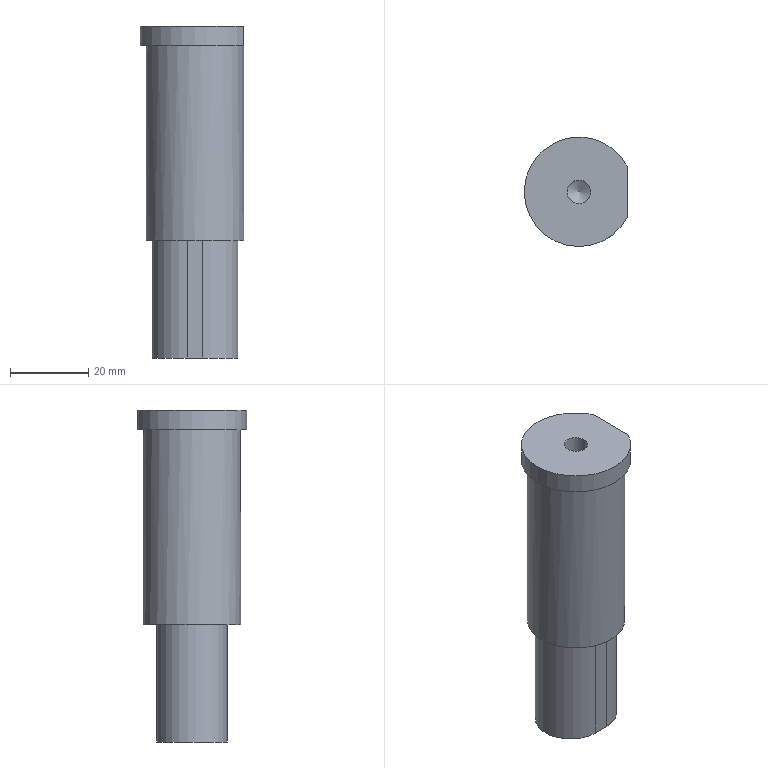Part | NX | features solid 2 | 1 solid | 15 faces | box 26.5 x 28 x 85 mm | volume 36969 mm3 | plane 7 | cylinder 7 | cone 1 | commonest cylinder face diameters 28 x3 18 x2 6 x1 25 x1
STEP:
#1=CARTESIAN_POINT('',(-212.5,0.005131,75.));
#2=VERTEX_POINT('',#1);
#3=CARTESIAN_POINT('',(-212.5,6.31,75.));
#4=VERTEX_POINT('',#3);
#5=CARTESIAN_POINT('',(-212.5,-22.334,75.));
#6=DIRECTION('',(0.,1.,0.));
#7=VECTOR('',#6,1000.);
#8=LINE('',#5,#7);
#9=EDGE_CURVE('',#2,#4,#8,.T.);
#10=ORIENTED_EDGE('',*,*,#9,.F.);
#11=CARTESIAN_POINT('',(-225.,0.005131,75.));
#12=DIRECTION('',(0.,0.,1.));
#13=DIRECTION('',(0.,-1.,0.));
#14=AXIS2_PLACEMENT_3D('',#11,#12,#13);
#15=CIRCLE('',#14,12.5);
#16=EDGE_CURVE('',#2,#2,#15,.T.);
#17=ORIENTED_EDGE('',*,*,#16,.T.);
#18=CARTESIAN_POINT('',(-212.5,-6.3,75.));
#19=VERTEX_POINT('',#18);
#20=CARTESIAN_POINT('',(-212.5,-22.334,75.));
#21=DIRECTION('',(0.,1.,0.));
#22=VECTOR('',#21,1000.);
#23=LINE('',#20,#22);
#24=EDGE_CURVE('',#19,#2,#23,.T.);
#25=ORIENTED_EDGE('',*,*,#24,.F.);
#26=CARTESIAN_POINT('',(-231.305,12.505,75.));
#27=VERTEX_POINT('',#26);
#28=CARTESIAN_POINT('',(-225.,0.005131,75.));
#29=DIRECTION('',(0.,0.,1.));
#30=DIRECTION('',(0.,-1.,0.));
#31=AXIS2_PLACEMENT_3D('',#28,#29,#30);
#32=CIRCLE('',#31,14.);
#33=EDGE_CURVE('',#27,#19,#32,.T.);
#34=ORIENTED_EDGE('',*,*,#33,.F.);
#35=CARTESIAN_POINT('',(-218.695,12.505,75.));
#36=VERTEX_POINT('',#35);
#37=CARTESIAN_POINT('',(-225.,0.005131,75.));
#38=DIRECTION('',(0.,0.,1.));
#39=DIRECTION('',(1.,0.,0.));
#40=AXIS2_PLACEMENT_3D('',#37,#38,#39);
#41=CIRCLE('',#40,14.);
#42=EDGE_CURVE('',#27,#36,#41,.F.);
#43=ORIENTED_EDGE('',*,*,#42,.T.);
#44=CARTESIAN_POINT('',(-225.,0.005131,75.));
#45=DIRECTION('',(0.,0.,1.));
#46=DIRECTION('',(0.,-1.,0.));
#47=AXIS2_PLACEMENT_3D('',#44,#45,#46);
#48=CIRCLE('',#47,14.);
#49=EDGE_CURVE('',#4,#36,#48,.T.);
#50=ORIENTED_EDGE('',*,*,#49,.F.);
#51=EDGE_LOOP('',(#10,#17,#25,#34,#43,#50));
#52=FACE_BOUND('',#51,.T.);
#53=CARTESIAN_POINT('',(-225.,0.005131,75.));
#54=DIRECTION('',(0.,0.,1.));
#55=DIRECTION('',(0.,-1.,0.));
#56=AXIS2_PLACEMENT_3D('',#53,#54,#55);
#57=PLANE('',#56);
#58=ADVANCED_FACE('',(#52),#57,.F.);
#59=CARTESIAN_POINT('',(-212.5,6.31,80.));
#60=VERTEX_POINT('',#59);
#61=CARTESIAN_POINT('',(-218.695,12.505,80.));
#62=VERTEX_POINT('',#61);
#63=CARTESIAN_POINT('',(-225.,0.005131,80.));
#64=DIRECTION('',(0.,0.,1.));
#65=DIRECTION('',(0.,-1.,0.));
#66=AXIS2_PLACEMENT_3D('',#63,#64,#65);
#67=CIRCLE('',#66,14.);
#68=EDGE_CURVE('',#60,#62,#67,.T.);
#69=ORIENTED_EDGE('',*,*,#68,.F.);
#70=CARTESIAN_POINT('',(-212.5,6.31,75.));
#71=DIRECTION('',(0.,0.,1.));
#72=VECTOR('',#71,1000.);
#73=LINE('',#70,#72);
#74=EDGE_CURVE('',#60,#4,#73,.F.);
#75=ORIENTED_EDGE('',*,*,#74,.T.);
#76=ORIENTED_EDGE('',*,*,#49,.T.);
#77=CARTESIAN_POINT('',(-218.695,12.505,83.));
#78=DIRECTION('',(0.,0.,-1.));
#79=VECTOR('',#78,1000.);
#80=LINE('',#77,#79);
#81=EDGE_CURVE('',#62,#36,#80,.T.);
#82=ORIENTED_EDGE('',*,*,#81,.F.);
#83=EDGE_LOOP('',(#69,#75,#76,#82));
#84=FACE_BOUND('',#83,.T.);
#85=CARTESIAN_POINT('',(-225.,0.005131,75.));
#86=DIRECTION('',(0.,0.,1.));
#87=DIRECTION('',(0.,-1.,0.));
#88=AXIS2_PLACEMENT_3D('',#85,#86,#87);
#89=CYLINDRICAL_SURFACE('',#88,14.);
#90=ADVANCED_FACE('',(#84),#89,.T.);
#91=ORIENTED_EDGE('',*,*,#33,.T.);
#92=CARTESIAN_POINT('',(-212.5,-6.3,80.));
#93=VERTEX_POINT('',#92);
#94=CARTESIAN_POINT('',(-212.5,-6.3,75.));
#95=DIRECTION('',(0.,0.,1.));
#96=VECTOR('',#95,1000.);
#97=LINE('',#94,#96);
#98=EDGE_CURVE('',#19,#93,#97,.T.);
#99=ORIENTED_EDGE('',*,*,#98,.T.);
#100=CARTESIAN_POINT('',(-231.305,12.505,80.));
#101=VERTEX_POINT('',#100);
#102=CARTESIAN_POINT('',(-225.,0.005131,80.));
#103=DIRECTION('',(0.,0.,1.));
#104=DIRECTION('',(0.,-1.,0.));
#105=AXIS2_PLACEMENT_3D('',#102,#103,#104);
#106=CIRCLE('',#105,14.);
#107=EDGE_CURVE('',#101,#93,#106,.T.);
#108=ORIENTED_EDGE('',*,*,#107,.F.);
#109=CARTESIAN_POINT('',(-231.305,12.505,83.));
#110=DIRECTION('',(0.,0.,-1.));
#111=VECTOR('',#110,1000.);
#112=LINE('',#109,#111);
#113=EDGE_CURVE('',#101,#27,#112,.T.);
#114=ORIENTED_EDGE('',*,*,#113,.T.);
#115=EDGE_LOOP('',(#91,#99,#108,#114));
#116=FACE_BOUND('',#115,.T.);
#117=CARTESIAN_POINT('',(-225.,0.005131,75.));
#118=DIRECTION('',(0.,0.,1.));
#119=DIRECTION('',(0.,-1.,0.));
#120=AXIS2_PLACEMENT_3D('',#117,#118,#119);
#121=CYLINDRICAL_SURFACE('',#120,14.);
#122=ADVANCED_FACE('',(#116),#121,.T.);
#123=CARTESIAN_POINT('',(-225.,3.005,80.));
#124=VERTEX_POINT('',#123);
#125=CARTESIAN_POINT('',(-225.,0.005131,80.));
#126=DIRECTION('',(0.,0.,-1.));
#127=DIRECTION('',(0.,1.,0.));
#128=AXIS2_PLACEMENT_3D('',#125,#126,#127);
#129=CIRCLE('',#128,3.);
#130=EDGE_CURVE('',#124,#124,#129,.T.);
#131=ORIENTED_EDGE('',*,*,#130,.T.);
#132=EDGE_LOOP('',(#131));
#133=FACE_BOUND('',#132,.T.);
#134=ORIENTED_EDGE('',*,*,#107,.T.);
#135=CARTESIAN_POINT('',(-212.5,-22.334,80.));
#136=DIRECTION('',(0.,1.,0.));
#137=VECTOR('',#136,1000.);
#138=LINE('',#135,#137);
#139=EDGE_CURVE('',#93,#60,#138,.T.);
#140=ORIENTED_EDGE('',*,*,#139,.T.);
#141=ORIENTED_EDGE('',*,*,#68,.T.);
#142=CARTESIAN_POINT('',(-225.,0.005131,80.));
#143=DIRECTION('',(0.,0.,1.));
#144=DIRECTION('',(1.,0.,0.));
#145=AXIS2_PLACEMENT_3D('',#142,#143,#144);
#146=CIRCLE('',#145,14.);
#147=EDGE_CURVE('',#101,#62,#146,.F.);
#148=ORIENTED_EDGE('',*,*,#147,.F.);
#149=EDGE_LOOP('',(#134,#140,#141,#148));
#150=FACE_BOUND('',#149,.T.);
#151=CARTESIAN_POINT('',(-225.,0.005131,80.));
#152=DIRECTION('',(0.,0.,1.));
#153=DIRECTION('',(0.,-1.,0.));
#154=AXIS2_PLACEMENT_3D('',#151,#152,#153);
#155=PLANE('',#154);
#156=ADVANCED_FACE('',(#133,#150),#155,.T.);
#157=CARTESIAN_POINT('',(-225.,-12.495,25.));
#158=VERTEX_POINT('',#157);
#159=CARTESIAN_POINT('',(-225.,0.005131,25.));
#160=DIRECTION('',(0.,0.,1.));
#161=DIRECTION('',(0.,-1.,0.));
#162=AXIS2_PLACEMENT_3D('',#159,#160,#161);
#163=CIRCLE('',#162,12.5);
#164=EDGE_CURVE('',#158,#158,#163,.T.);
#165=ORIENTED_EDGE('',*,*,#164,.F.);
#166=EDGE_LOOP('',(#165));
#167=FACE_BOUND('',#166,.T.);
#168=CARTESIAN_POINT('',(-223.,-8.995,25.));
#169=VERTEX_POINT('',#168);
#170=CARTESIAN_POINT('',(-227.,-8.995,25.));
#171=VERTEX_POINT('',#170);
#172=CARTESIAN_POINT('',(-225.,-8.995,25.));
#173=DIRECTION('',(-1.,0.,0.));
#174=VECTOR('',#173,1000.);
#175=LINE('',#172,#174);
#176=EDGE_CURVE('',#169,#171,#175,.T.);
#177=ORIENTED_EDGE('',*,*,#176,.F.);
#178=CARTESIAN_POINT('',(-223.,9.005,25.));
#179=VERTEX_POINT('',#178);
#180=CARTESIAN_POINT('',(-223.,0.005131,25.));
#181=DIRECTION('',(0.,0.,1.));
#182=DIRECTION('',(0.,-1.,0.));
#183=AXIS2_PLACEMENT_3D('',#180,#181,#182);
#184=CIRCLE('',#183,9.);
#185=EDGE_CURVE('',#169,#179,#184,.T.);
#186=ORIENTED_EDGE('',*,*,#185,.T.);
#187=CARTESIAN_POINT('',(-227.,9.005,25.));
#188=VERTEX_POINT('',#187);
#189=CARTESIAN_POINT('',(-225.,9.005,25.));
#190=DIRECTION('',(-1.,0.,0.));
#191=VECTOR('',#190,1000.);
#192=LINE('',#189,#191);
#193=EDGE_CURVE('',#179,#188,#192,.T.);
#194=ORIENTED_EDGE('',*,*,#193,.T.);
#195=CARTESIAN_POINT('',(-227.,0.005131,25.));
#196=DIRECTION('',(0.,0.,1.));
#197=DIRECTION('',(0.,-1.,0.));
#198=AXIS2_PLACEMENT_3D('',#195,#196,#197);
#199=CIRCLE('',#198,9.);
#200=EDGE_CURVE('',#188,#171,#199,.T.);
#201=ORIENTED_EDGE('',*,*,#200,.T.);
#202=EDGE_LOOP('',(#177,#186,#194,#201));
#203=FACE_BOUND('',#202,.T.);
#204=CARTESIAN_POINT('',(-225.,0.005131,25.));
#205=DIRECTION('',(0.,0.,1.));
#206=DIRECTION('',(0.,-1.,0.));
#207=AXIS2_PLACEMENT_3D('',#204,#205,#206);
#208=PLANE('',#207);
#209=ADVANCED_FACE('',(#167,#203),#208,.F.);
#210=ORIENTED_EDGE('',*,*,#164,.T.);
#211=EDGE_LOOP('',(#210));
#212=FACE_BOUND('',#211,.T.);
#213=ORIENTED_EDGE('',*,*,#16,.F.);
#214=EDGE_LOOP('',(#213));
#215=FACE_BOUND('',#214,.T.);
#216=CARTESIAN_POINT('',(-225.,0.005131,80.));
#217=DIRECTION('',(0.,0.,-1.));
#218=DIRECTION('',(0.,1.,0.));
#219=AXIS2_PLACEMENT_3D('',#216,#217,#218);
#220=CYLINDRICAL_SURFACE('',#219,12.5);
#221=ADVANCED_FACE('',(#212,#215),#220,.T.);
#222=ORIENTED_EDGE('',*,*,#113,.F.);
#223=ORIENTED_EDGE('',*,*,#147,.T.);
#224=ORIENTED_EDGE('',*,*,#81,.T.);
#225=ORIENTED_EDGE('',*,*,#42,.F.);
#226=EDGE_LOOP('',(#222,#223,#224,#225));
#227=FACE_BOUND('',#226,.T.);
#228=CARTESIAN_POINT('',(-225.,0.005131,75.));
#229=DIRECTION('',(0.,0.,1.));
#230=DIRECTION('',(0.,-1.,0.));
#231=AXIS2_PLACEMENT_3D('',#228,#229,#230);
#232=CYLINDRICAL_SURFACE('',#231,14.);
#233=ADVANCED_FACE('',(#227),#232,.T.);
#234=CARTESIAN_POINT('',(-223.,-8.995,-5.));
#235=VERTEX_POINT('',#234);
#236=CARTESIAN_POINT('',(-223.,-8.995,0.));
#237=DIRECTION('',(0.,0.,1.));
#238=VECTOR('',#237,1000.);
#239=LINE('',#236,#238);
#240=EDGE_CURVE('',#235,#169,#239,.T.);
#241=ORIENTED_EDGE('',*,*,#240,.T.);
#242=ORIENTED_EDGE('',*,*,#176,.T.);
#243=CARTESIAN_POINT('',(-227.,-8.995,-5.));
#244=VERTEX_POINT('',#243);
#245=CARTESIAN_POINT('',(-227.,-8.995,0.));
#246=DIRECTION('',(0.,0.,1.));
#247=VECTOR('',#246,1000.);
#248=LINE('',#245,#247);
#249=EDGE_CURVE('',#244,#171,#248,.T.);
#250=ORIENTED_EDGE('',*,*,#249,.F.);
#251=CARTESIAN_POINT('',(-227.,-8.995,-5.));
#252=DIRECTION('',(-1.,0.,0.));
#253=VECTOR('',#252,1000.);
#254=LINE('',#251,#253);
#255=EDGE_CURVE('',#235,#244,#254,.T.);
#256=ORIENTED_EDGE('',*,*,#255,.F.);
#257=EDGE_LOOP('',(#241,#242,#250,#256));
#258=FACE_BOUND('',#257,.T.);
#259=CARTESIAN_POINT('',(-223.,-8.995,0.));
#260=DIRECTION('',(0.,1.,0.));
#261=DIRECTION('',(0.,0.,1.));
#262=AXIS2_PLACEMENT_3D('',#259,#260,#261);
#263=PLANE('',#262);
#264=ADVANCED_FACE('',(#258),#263,.F.);
#265=ORIENTED_EDGE('',*,*,#200,.F.);
#266=CARTESIAN_POINT('',(-227.,9.005,-5.));
#267=VERTEX_POINT('',#266);
#268=CARTESIAN_POINT('',(-227.,9.005,0.));
#269=DIRECTION('',(0.,0.,1.));
#270=VECTOR('',#269,1000.);
#271=LINE('',#268,#270);
#272=EDGE_CURVE('',#267,#188,#271,.T.);
#273=ORIENTED_EDGE('',*,*,#272,.F.);
#274=CARTESIAN_POINT('',(-227.,0.005131,-5.));
#275=DIRECTION('',(0.,0.,1.));
#276=DIRECTION('',(0.,-1.,0.));
#277=AXIS2_PLACEMENT_3D('',#274,#275,#276);
#278=CIRCLE('',#277,9.);
#279=EDGE_CURVE('',#267,#244,#278,.T.);
#280=ORIENTED_EDGE('',*,*,#279,.T.);
#281=ORIENTED_EDGE('',*,*,#249,.T.);
#282=EDGE_LOOP('',(#265,#273,#280,#281));
#283=FACE_BOUND('',#282,.T.);
#284=CARTESIAN_POINT('',(-227.,0.005131,0.));
#285=DIRECTION('',(0.,0.,1.));
#286=DIRECTION('',(0.,-1.,0.));
#287=AXIS2_PLACEMENT_3D('',#284,#285,#286);
#288=CYLINDRICAL_SURFACE('',#287,9.);
#289=ADVANCED_FACE('',(#283),#288,.T.);
#290=ORIENTED_EDGE('',*,*,#193,.F.);
#291=CARTESIAN_POINT('',(-223.,9.005,-5.));
#292=VERTEX_POINT('',#291);
#293=CARTESIAN_POINT('',(-223.,9.005,0.));
#294=DIRECTION('',(0.,0.,1.));
#295=VECTOR('',#294,1000.);
#296=LINE('',#293,#295);
#297=EDGE_CURVE('',#292,#179,#296,.T.);
#298=ORIENTED_EDGE('',*,*,#297,.F.);
#299=CARTESIAN_POINT('',(-227.,9.005,-5.));
#300=DIRECTION('',(-1.,0.,0.));
#301=VECTOR('',#300,1000.);
#302=LINE('',#299,#301);
#303=EDGE_CURVE('',#292,#267,#302,.T.);
#304=ORIENTED_EDGE('',*,*,#303,.T.);
#305=ORIENTED_EDGE('',*,*,#272,.T.);
#306=EDGE_LOOP('',(#290,#298,#304,#305));
#307=FACE_BOUND('',#306,.T.);
#308=CARTESIAN_POINT('',(-223.,9.005,0.));
#309=DIRECTION('',(0.,1.,0.));
#310=DIRECTION('',(0.,0.,1.));
#311=AXIS2_PLACEMENT_3D('',#308,#309,#310);
#312=PLANE('',#311);
#313=ADVANCED_FACE('',(#307),#312,.T.);
#314=ORIENTED_EDGE('',*,*,#185,.F.);
#315=ORIENTED_EDGE('',*,*,#240,.F.);
#316=CARTESIAN_POINT('',(-223.,0.005131,-5.));
#317=DIRECTION('',(0.,0.,1.));
#318=DIRECTION('',(0.,-1.,0.));
#319=AXIS2_PLACEMENT_3D('',#316,#317,#318);
#320=CIRCLE('',#319,9.);
#321=EDGE_CURVE('',#235,#292,#320,.T.);
#322=ORIENTED_EDGE('',*,*,#321,.T.);
#323=ORIENTED_EDGE('',*,*,#297,.T.);
#324=EDGE_LOOP('',(#314,#315,#322,#323));
#325=FACE_BOUND('',#324,.T.);
#326=CARTESIAN_POINT('',(-223.,0.005131,0.));
#327=DIRECTION('',(0.,0.,1.));
#328=DIRECTION('',(0.,-1.,0.));
#329=AXIS2_PLACEMENT_3D('',#326,#327,#328);
#330=CYLINDRICAL_SURFACE('',#329,9.);
#331=ADVANCED_FACE('',(#325),#330,.T.);
#332=ORIENTED_EDGE('',*,*,#255,.T.);
#333=ORIENTED_EDGE('',*,*,#279,.F.);
#334=ORIENTED_EDGE('',*,*,#303,.F.);
#335=ORIENTED_EDGE('',*,*,#321,.F.);
#336=EDGE_LOOP('',(#332,#333,#334,#335));
#337=FACE_BOUND('',#336,.T.);
#338=CARTESIAN_POINT('',(-227.,0.005131,-5.));
#339=DIRECTION('',(0.,0.,1.));
#340=DIRECTION('',(0.,-1.,0.));
#341=AXIS2_PLACEMENT_3D('',#338,#339,#340);
#342=PLANE('',#341);
#343=ADVANCED_FACE('',(#337),#342,.F.);
#344=CARTESIAN_POINT('',(-225.,3.005,67.));
#345=VERTEX_POINT('',#344);
#346=CARTESIAN_POINT('',(-225.,0.005131,67.));
#347=DIRECTION('',(0.,0.,-1.));
#348=DIRECTION('',(0.,1.,0.));
#349=AXIS2_PLACEMENT_3D('',#346,#347,#348);
#350=CIRCLE('',#349,3.);
#351=EDGE_CURVE('',#345,#345,#350,.T.);
#352=ORIENTED_EDGE('',*,*,#351,.F.);
#353=EDGE_LOOP('',(#352));
#354=FACE_BOUND('',#353,.T.);
#355=CARTESIAN_POINT('',(-225.,0.005131,65.268));
#356=VERTEX_POINT('',#355);
#357=VERTEX_LOOP('',#356);
#358=FACE_BOUND('',#357,.T.);
#359=CARTESIAN_POINT('',(-225.,0.005131,67.));
#360=DIRECTION('',(0.,0.,1.));
#361=DIRECTION('',(0.,-1.,0.));
#362=AXIS2_PLACEMENT_3D('',#359,#360,#361);
#363=CONICAL_SURFACE('',#362,3.,1.047);
#364=ADVANCED_FACE('',(#354,#358),#363,.F.);
#365=ORIENTED_EDGE('',*,*,#351,.T.);
#366=EDGE_LOOP('',(#365));
#367=FACE_BOUND('',#366,.T.);
#368=ORIENTED_EDGE('',*,*,#130,.F.);
#369=EDGE_LOOP('',(#368));
#370=FACE_BOUND('',#369,.T.);
#371=CARTESIAN_POINT('',(-225.,0.005131,80.));
#372=DIRECTION('',(0.,0.,-1.));
#373=DIRECTION('',(0.,1.,0.));
#374=AXIS2_PLACEMENT_3D('',#371,#372,#373);
#375=CYLINDRICAL_SURFACE('',#374,3.);
#376=ADVANCED_FACE('',(#367,#370),#375,.F.);
#377=ORIENTED_EDGE('',*,*,#139,.F.);
#378=ORIENTED_EDGE('',*,*,#98,.F.);
#379=ORIENTED_EDGE('',*,*,#24,.T.);
#380=ORIENTED_EDGE('',*,*,#9,.T.);
#381=ORIENTED_EDGE('',*,*,#74,.F.);
#382=EDGE_LOOP('',(#377,#378,#379,#380,#381));
#383=FACE_BOUND('',#382,.T.);
#384=CARTESIAN_POINT('',(-212.5,-22.334,75.));
#385=DIRECTION('',(1.,0.,0.));
#386=DIRECTION('',(0.,1.,0.));
#387=AXIS2_PLACEMENT_3D('',#384,#385,#386);
#388=PLANE('',#387);
#389=ADVANCED_FACE('',(#383),#388,.T.);
#390=CLOSED_SHELL('',(#58,#90,#122,#156,#209,#221,#233,#264,#289,#313,#331,#343,#364,#376,#389));
#391=MANIFOLD_SOLID_BREP('',#390);
#392=(LENGTH_UNIT()NAMED_UNIT(*)SI_UNIT(.MILLI.,.METRE.));
#393=UNCERTAINTY_MEASURE_WITH_UNIT(LENGTH_MEASURE(0.00001),#392,'','');
#394=(NAMED_UNIT(*)PLANE_ANGLE_UNIT()SI_UNIT($,.RADIAN.));
#395=(NAMED_UNIT(*)SI_UNIT($,.STERADIAN.)SOLID_ANGLE_UNIT());
#396=(GEOMETRIC_REPRESENTATION_CONTEXT(3)GLOBAL_UNCERTAINTY_ASSIGNED_CONTEXT((#393))GLOBAL_UNIT_ASSIGNED_CONTEXT((#392,#394,#395))REPRESENTATION_CONTEXT('',''));
#397=ADVANCED_BREP_SHAPE_REPRESENTATION('',(#391),#396);